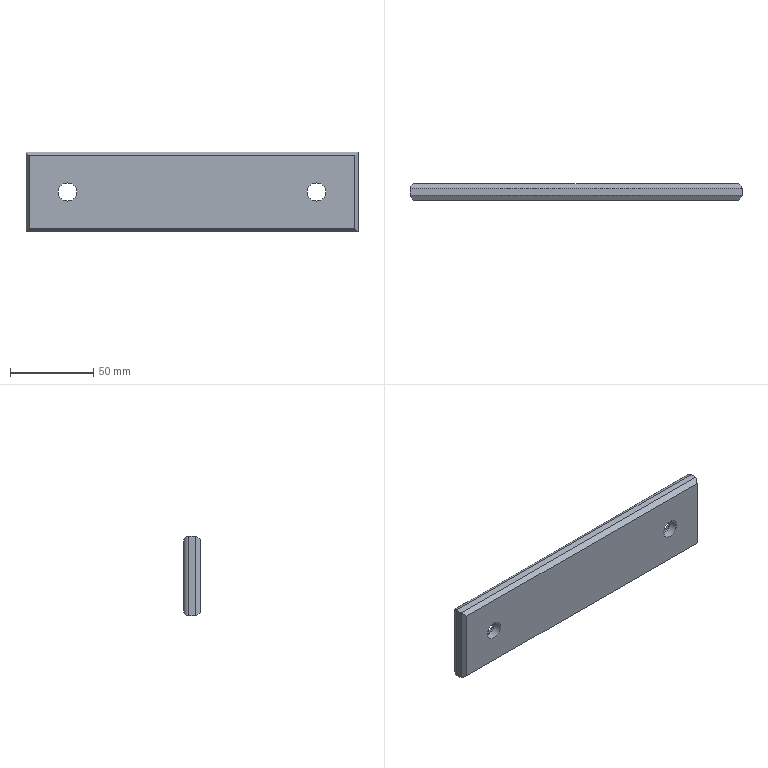Part | NX | features solid 2 | 1 solid | 22 faces | box 200 x 10 x 48 mm | volume 90126 mm3 | plane 12 | cylinder 8 | torus 2 | commonest cylinder face diameters 6 x4 11 x2 17.5 x2
STEP:
#1=CARTESIAN_POINT('',(310.,367.,141.));
#2=VERTEX_POINT('',#1);
#3=CARTESIAN_POINT('',(310.,363.,141.));
#4=VERTEX_POINT('',#3);
#5=CARTESIAN_POINT('',(310.,370.,141.));
#6=DIRECTION('',(0.,-1.,0.));
#7=VECTOR('',#6,1000.);
#8=LINE('',#5,#7);
#9=EDGE_CURVE('',#2,#4,#8,.T.);
#10=ORIENTED_EDGE('',*,*,#9,.T.);
#11=CARTESIAN_POINT('',(110.,363.,141.));
#12=VERTEX_POINT('',#11);
#13=CARTESIAN_POINT('',(110.,363.,141.));
#14=DIRECTION('',(-1.,0.,0.));
#15=VECTOR('',#14,1000.);
#16=LINE('',#13,#15);
#17=EDGE_CURVE('',#4,#12,#16,.T.);
#18=ORIENTED_EDGE('',*,*,#17,.T.);
#19=CARTESIAN_POINT('',(110.,367.,141.));
#20=VERTEX_POINT('',#19);
#21=CARTESIAN_POINT('',(110.,370.,141.));
#22=DIRECTION('',(0.,-1.,0.));
#23=VECTOR('',#22,1000.);
#24=LINE('',#21,#23);
#25=EDGE_CURVE('',#20,#12,#24,.T.);
#26=ORIENTED_EDGE('',*,*,#25,.F.);
#27=CARTESIAN_POINT('',(310.,367.,141.));
#28=DIRECTION('',(-1.,0.,0.));
#29=VECTOR('',#28,1000.);
#30=LINE('',#27,#29);
#31=EDGE_CURVE('',#20,#2,#30,.F.);
#32=ORIENTED_EDGE('',*,*,#31,.T.);
#33=EDGE_LOOP('',(#10,#18,#26,#32));
#34=FACE_BOUND('',#33,.T.);
#35=CARTESIAN_POINT('',(310.,370.,141.));
#36=DIRECTION('',(0.,0.,1.));
#37=DIRECTION('',(-1.,0.,0.));
#38=AXIS2_PLACEMENT_3D('',#35,#36,#37);
#39=PLANE('',#38);
#40=ADVANCED_FACE('',(#34),#39,.F.);
#41=ORIENTED_EDGE('',*,*,#25,.T.);
#42=CARTESIAN_POINT('',(110.,363.,189.));
#43=VERTEX_POINT('',#42);
#44=CARTESIAN_POINT('',(110.,363.,190.));
#45=DIRECTION('',(0.,0.,1.));
#46=VECTOR('',#45,1000.);
#47=LINE('',#44,#46);
#48=EDGE_CURVE('',#12,#43,#47,.T.);
#49=ORIENTED_EDGE('',*,*,#48,.T.);
#50=CARTESIAN_POINT('',(110.,367.,189.));
#51=VERTEX_POINT('',#50);
#52=CARTESIAN_POINT('',(110.,370.,189.));
#53=DIRECTION('',(0.,-1.,0.));
#54=VECTOR('',#53,1000.);
#55=LINE('',#52,#54);
#56=EDGE_CURVE('',#51,#43,#55,.T.);
#57=ORIENTED_EDGE('',*,*,#56,.F.);
#58=CARTESIAN_POINT('',(110.,367.,141.));
#59=DIRECTION('',(0.,0.,-1.));
#60=VECTOR('',#59,1000.);
#61=LINE('',#58,#60);
#62=EDGE_CURVE('',#51,#20,#61,.T.);
#63=ORIENTED_EDGE('',*,*,#62,.T.);
#64=EDGE_LOOP('',(#41,#49,#57,#63));
#65=FACE_BOUND('',#64,.T.);
#66=CARTESIAN_POINT('',(110.,370.,190.));
#67=DIRECTION('',(-1.,0.,0.));
#68=DIRECTION('',(0.,0.,-1.));
#69=AXIS2_PLACEMENT_3D('',#66,#67,#68);
#70=PLANE('',#69);
#71=ADVANCED_FACE('',(#65),#70,.T.);
#72=ORIENTED_EDGE('',*,*,#56,.T.);
#73=CARTESIAN_POINT('',(310.,363.,189.));
#74=VERTEX_POINT('',#73);
#75=CARTESIAN_POINT('',(310.,363.,189.));
#76=DIRECTION('',(1.,0.,0.));
#77=VECTOR('',#76,1000.);
#78=LINE('',#75,#77);
#79=EDGE_CURVE('',#43,#74,#78,.T.);
#80=ORIENTED_EDGE('',*,*,#79,.T.);
#81=CARTESIAN_POINT('',(310.,367.,189.));
#82=VERTEX_POINT('',#81);
#83=CARTESIAN_POINT('',(310.,370.,189.));
#84=DIRECTION('',(0.,-1.,0.));
#85=VECTOR('',#84,1000.);
#86=LINE('',#83,#85);
#87=EDGE_CURVE('',#82,#74,#86,.T.);
#88=ORIENTED_EDGE('',*,*,#87,.F.);
#89=CARTESIAN_POINT('',(110.,367.,189.));
#90=DIRECTION('',(-1.,0.,0.));
#91=VECTOR('',#90,1000.);
#92=LINE('',#89,#91);
#93=EDGE_CURVE('',#82,#51,#92,.T.);
#94=ORIENTED_EDGE('',*,*,#93,.T.);
#95=EDGE_LOOP('',(#72,#80,#88,#94));
#96=FACE_BOUND('',#95,.T.);
#97=CARTESIAN_POINT('',(310.,370.,189.));
#98=DIRECTION('',(0.,0.,1.));
#99=DIRECTION('',(-1.,0.,0.));
#100=AXIS2_PLACEMENT_3D('',#97,#98,#99);
#101=PLANE('',#100);
#102=ADVANCED_FACE('',(#96),#101,.T.);
#103=ORIENTED_EDGE('',*,*,#87,.T.);
#104=CARTESIAN_POINT('',(310.,363.,141.));
#105=DIRECTION('',(0.,0.,-1.));
#106=VECTOR('',#105,1000.);
#107=LINE('',#104,#106);
#108=EDGE_CURVE('',#74,#4,#107,.T.);
#109=ORIENTED_EDGE('',*,*,#108,.T.);
#110=ORIENTED_EDGE('',*,*,#9,.F.);
#111=CARTESIAN_POINT('',(310.,367.,190.));
#112=DIRECTION('',(0.,0.,-1.));
#113=VECTOR('',#112,1000.);
#114=LINE('',#111,#113);
#115=EDGE_CURVE('',#2,#82,#114,.F.);
#116=ORIENTED_EDGE('',*,*,#115,.T.);
#117=EDGE_LOOP('',(#103,#109,#110,#116));
#118=FACE_BOUND('',#117,.T.);
#119=CARTESIAN_POINT('',(310.,370.,190.));
#120=DIRECTION('',(-1.,0.,0.));
#121=DIRECTION('',(0.,0.,-1.));
#122=AXIS2_PLACEMENT_3D('',#119,#120,#121);
#123=PLANE('',#122);
#124=ADVANCED_FACE('',(#118),#123,.F.);
#125=CARTESIAN_POINT('',(113.,370.,186.));
#126=VERTEX_POINT('',#125);
#127=CARTESIAN_POINT('',(307.,370.,186.));
#128=VERTEX_POINT('',#127);
#129=CARTESIAN_POINT('',(310.,370.,186.));
#130=DIRECTION('',(-1.,0.,0.));
#131=VECTOR('',#130,1000.);
#132=LINE('',#129,#131);
#133=EDGE_CURVE('',#126,#128,#132,.F.);
#134=ORIENTED_EDGE('',*,*,#133,.T.);
#135=CARTESIAN_POINT('',(307.,370.,144.));
#136=VERTEX_POINT('',#135);
#137=CARTESIAN_POINT('',(307.,370.,190.));
#138=DIRECTION('',(0.,0.,-1.));
#139=VECTOR('',#138,1000.);
#140=LINE('',#137,#139);
#141=EDGE_CURVE('',#128,#136,#140,.T.);
#142=ORIENTED_EDGE('',*,*,#141,.T.);
#143=CARTESIAN_POINT('',(113.,370.,144.));
#144=VERTEX_POINT('',#143);
#145=CARTESIAN_POINT('',(310.,370.,144.));
#146=DIRECTION('',(-1.,0.,0.));
#147=VECTOR('',#146,1000.);
#148=LINE('',#145,#147);
#149=EDGE_CURVE('',#136,#144,#148,.T.);
#150=ORIENTED_EDGE('',*,*,#149,.T.);
#151=CARTESIAN_POINT('',(113.,370.,189.));
#152=DIRECTION('',(0.,0.,-1.));
#153=VECTOR('',#152,1000.);
#154=LINE('',#151,#153);
#155=EDGE_CURVE('',#144,#126,#154,.F.);
#156=ORIENTED_EDGE('',*,*,#155,.T.);
#157=EDGE_LOOP('',(#134,#142,#150,#156));
#158=FACE_BOUND('',#157,.T.);
#159=CARTESIAN_POINT('',(285.,370.,154.25));
#160=VERTEX_POINT('',#159);
#161=CARTESIAN_POINT('',(285.,370.,165.));
#162=DIRECTION('',(0.,-1.,0.));
#163=DIRECTION('',(0.,0.,-1.));
#164=AXIS2_PLACEMENT_3D('',#161,#162,#163);
#165=CIRCLE('',#164,10.75);
#166=EDGE_CURVE('',#160,#160,#165,.T.);
#167=ORIENTED_EDGE('',*,*,#166,.T.);
#168=EDGE_LOOP('',(#167));
#169=FACE_BOUND('',#168,.T.);
#170=CARTESIAN_POINT('',(135.,370.,154.25));
#171=VERTEX_POINT('',#170);
#172=CARTESIAN_POINT('',(135.,370.,165.));
#173=DIRECTION('',(0.,-1.,0.));
#174=DIRECTION('',(0.,0.,-1.));
#175=AXIS2_PLACEMENT_3D('',#172,#173,#174);
#176=CIRCLE('',#175,10.75);
#177=EDGE_CURVE('',#171,#171,#176,.T.);
#178=ORIENTED_EDGE('',*,*,#177,.T.);
#179=EDGE_LOOP('',(#178));
#180=FACE_BOUND('',#179,.T.);
#181=CARTESIAN_POINT('',(310.,370.,190.));
#182=DIRECTION('',(0.,-1.,0.));
#183=DIRECTION('',(0.,0.,-1.));
#184=AXIS2_PLACEMENT_3D('',#181,#182,#183);
#185=PLANE('',#184);
#186=ADVANCED_FACE('',(#158,#169,#180),#185,.F.);
#187=CARTESIAN_POINT('',(112.,360.,143.));
#188=VERTEX_POINT('',#187);
#189=CARTESIAN_POINT('',(308.,360.,143.));
#190=VERTEX_POINT('',#189);
#191=CARTESIAN_POINT('',(310.,360.,143.));
#192=DIRECTION('',(1.,0.,0.));
#193=VECTOR('',#192,1000.);
#194=LINE('',#191,#193);
#195=EDGE_CURVE('',#188,#190,#194,.T.);
#196=ORIENTED_EDGE('',*,*,#195,.T.);
#197=CARTESIAN_POINT('',(308.,360.,187.));
#198=VERTEX_POINT('',#197);
#199=CARTESIAN_POINT('',(308.,360.,189.));
#200=DIRECTION('',(0.,0.,1.));
#201=VECTOR('',#200,1000.);
#202=LINE('',#199,#201);
#203=EDGE_CURVE('',#190,#198,#202,.T.);
#204=ORIENTED_EDGE('',*,*,#203,.T.);
#205=CARTESIAN_POINT('',(112.,360.,187.));
#206=VERTEX_POINT('',#205);
#207=CARTESIAN_POINT('',(310.,360.,187.));
#208=DIRECTION('',(-1.,0.,0.));
#209=VECTOR('',#208,1000.);
#210=LINE('',#207,#209);
#211=EDGE_CURVE('',#198,#206,#210,.T.);
#212=ORIENTED_EDGE('',*,*,#211,.T.);
#213=CARTESIAN_POINT('',(112.,360.,190.));
#214=DIRECTION('',(0.,0.,-1.));
#215=VECTOR('',#214,1000.);
#216=LINE('',#213,#215);
#217=EDGE_CURVE('',#206,#188,#216,.T.);
#218=ORIENTED_EDGE('',*,*,#217,.T.);
#219=EDGE_LOOP('',(#196,#204,#212,#218));
#220=FACE_BOUND('',#219,.T.);
#221=CARTESIAN_POINT('',(135.,360.,159.5));
#222=VERTEX_POINT('',#221);
#223=CARTESIAN_POINT('',(135.,360.,165.));
#224=DIRECTION('',(0.,-1.,0.));
#225=DIRECTION('',(0.,0.,-1.));
#226=AXIS2_PLACEMENT_3D('',#223,#224,#225);
#227=CIRCLE('',#226,5.5);
#228=EDGE_CURVE('',#222,#222,#227,.T.);
#229=ORIENTED_EDGE('',*,*,#228,.F.);
#230=EDGE_LOOP('',(#229));
#231=FACE_BOUND('',#230,.T.);
#232=CARTESIAN_POINT('',(285.,360.,159.5));
#233=VERTEX_POINT('',#232);
#234=CARTESIAN_POINT('',(285.,360.,165.));
#235=DIRECTION('',(0.,-1.,0.));
#236=DIRECTION('',(0.,0.,-1.));
#237=AXIS2_PLACEMENT_3D('',#234,#235,#236);
#238=CIRCLE('',#237,5.5);
#239=EDGE_CURVE('',#233,#233,#238,.T.);
#240=ORIENTED_EDGE('',*,*,#239,.F.);
#241=EDGE_LOOP('',(#240));
#242=FACE_BOUND('',#241,.T.);
#243=CARTESIAN_POINT('',(310.,360.,190.));
#244=DIRECTION('',(0.,-1.,0.));
#245=DIRECTION('',(0.,0.,-1.));
#246=AXIS2_PLACEMENT_3D('',#243,#244,#245);
#247=PLANE('',#246);
#248=ADVANCED_FACE('',(#220,#231,#242),#247,.T.);
#249=ORIENTED_EDGE('',*,*,#239,.T.);
#250=EDGE_LOOP('',(#249));
#251=FACE_BOUND('',#250,.T.);
#252=CARTESIAN_POINT('',(285.,365.,159.5));
#253=VERTEX_POINT('',#252);
#254=CARTESIAN_POINT('',(285.,365.,165.));
#255=DIRECTION('',(0.,-1.,0.));
#256=DIRECTION('',(0.,0.,-1.));
#257=AXIS2_PLACEMENT_3D('',#254,#255,#256);
#258=CIRCLE('',#257,5.5);
#259=EDGE_CURVE('',#253,#253,#258,.T.);
#260=ORIENTED_EDGE('',*,*,#259,.F.);
#261=EDGE_LOOP('',(#260));
#262=FACE_BOUND('',#261,.T.);
#263=CARTESIAN_POINT('',(285.,360.,165.));
#264=DIRECTION('',(0.,-1.,0.));
#265=DIRECTION('',(0.,0.,-1.));
#266=AXIS2_PLACEMENT_3D('',#263,#264,#265);
#267=CYLINDRICAL_SURFACE('',#266,5.5);
#268=ADVANCED_FACE('',(#251,#262),#267,.F.);
#269=ORIENTED_EDGE('',*,*,#259,.T.);
#270=EDGE_LOOP('',(#269));
#271=FACE_BOUND('',#270,.T.);
#272=CARTESIAN_POINT('',(285.,365.,156.25));
#273=VERTEX_POINT('',#272);
#274=CARTESIAN_POINT('',(285.,365.,165.));
#275=DIRECTION('',(0.,-1.,0.));
#276=DIRECTION('',(0.,0.,-1.));
#277=AXIS2_PLACEMENT_3D('',#274,#275,#276);
#278=CIRCLE('',#277,8.75);
#279=EDGE_CURVE('',#273,#273,#278,.T.);
#280=ORIENTED_EDGE('',*,*,#279,.F.);
#281=EDGE_LOOP('',(#280));
#282=FACE_BOUND('',#281,.T.);
#283=CARTESIAN_POINT('',(285.,365.,165.));
#284=DIRECTION('',(0.,-1.,0.));
#285=DIRECTION('',(0.,0.,-1.));
#286=AXIS2_PLACEMENT_3D('',#283,#284,#285);
#287=PLANE('',#286);
#288=ADVANCED_FACE('',(#271,#282),#287,.F.);
#289=CARTESIAN_POINT('',(285.,368.,156.25));
#290=VERTEX_POINT('',#289);
#291=CARTESIAN_POINT('',(285.,368.,165.));
#292=DIRECTION('',(0.,-1.,0.));
#293=DIRECTION('',(0.,0.,-1.));
#294=AXIS2_PLACEMENT_3D('',#291,#292,#293);
#295=CIRCLE('',#294,8.75);
#296=EDGE_CURVE('',#290,#290,#295,.F.);
#297=ORIENTED_EDGE('',*,*,#296,.T.);
#298=EDGE_LOOP('',(#297));
#299=FACE_BOUND('',#298,.T.);
#300=ORIENTED_EDGE('',*,*,#279,.T.);
#301=EDGE_LOOP('',(#300));
#302=FACE_BOUND('',#301,.T.);
#303=CARTESIAN_POINT('',(285.,370.,165.));
#304=DIRECTION('',(0.,-1.,0.));
#305=DIRECTION('',(0.,0.,-1.));
#306=AXIS2_PLACEMENT_3D('',#303,#304,#305);
#307=CYLINDRICAL_SURFACE('',#306,8.75);
#308=ADVANCED_FACE('',(#299,#302),#307,.F.);
#309=ORIENTED_EDGE('',*,*,#228,.T.);
#310=EDGE_LOOP('',(#309));
#311=FACE_BOUND('',#310,.T.);
#312=CARTESIAN_POINT('',(135.,365.,159.5));
#313=VERTEX_POINT('',#312);
#314=CARTESIAN_POINT('',(135.,365.,165.));
#315=DIRECTION('',(0.,-1.,0.));
#316=DIRECTION('',(0.,0.,-1.));
#317=AXIS2_PLACEMENT_3D('',#314,#315,#316);
#318=CIRCLE('',#317,5.5);
#319=EDGE_CURVE('',#313,#313,#318,.T.);
#320=ORIENTED_EDGE('',*,*,#319,.F.);
#321=EDGE_LOOP('',(#320));
#322=FACE_BOUND('',#321,.T.);
#323=CARTESIAN_POINT('',(135.,360.,165.));
#324=DIRECTION('',(0.,-1.,0.));
#325=DIRECTION('',(0.,0.,-1.));
#326=AXIS2_PLACEMENT_3D('',#323,#324,#325);
#327=CYLINDRICAL_SURFACE('',#326,5.5);
#328=ADVANCED_FACE('',(#311,#322),#327,.F.);
#329=ORIENTED_EDGE('',*,*,#319,.T.);
#330=EDGE_LOOP('',(#329));
#331=FACE_BOUND('',#330,.T.);
#332=CARTESIAN_POINT('',(135.,365.,156.25));
#333=VERTEX_POINT('',#332);
#334=CARTESIAN_POINT('',(135.,365.,165.));
#335=DIRECTION('',(0.,-1.,0.));
#336=DIRECTION('',(0.,0.,-1.));
#337=AXIS2_PLACEMENT_3D('',#334,#335,#336);
#338=CIRCLE('',#337,8.75);
#339=EDGE_CURVE('',#333,#333,#338,.T.);
#340=ORIENTED_EDGE('',*,*,#339,.F.);
#341=EDGE_LOOP('',(#340));
#342=FACE_BOUND('',#341,.T.);
#343=CARTESIAN_POINT('',(135.,365.,165.));
#344=DIRECTION('',(0.,-1.,0.));
#345=DIRECTION('',(0.,0.,-1.));
#346=AXIS2_PLACEMENT_3D('',#343,#344,#345);
#347=PLANE('',#346);
#348=ADVANCED_FACE('',(#331,#342),#347,.F.);
#349=CARTESIAN_POINT('',(135.,368.,156.25));
#350=VERTEX_POINT('',#349);
#351=CARTESIAN_POINT('',(135.,368.,165.));
#352=DIRECTION('',(0.,-1.,0.));
#353=DIRECTION('',(0.,0.,-1.));
#354=AXIS2_PLACEMENT_3D('',#351,#352,#353);
#355=CIRCLE('',#354,8.75);
#356=EDGE_CURVE('',#350,#350,#355,.F.);
#357=ORIENTED_EDGE('',*,*,#356,.T.);
#358=EDGE_LOOP('',(#357));
#359=FACE_BOUND('',#358,.T.);
#360=ORIENTED_EDGE('',*,*,#339,.T.);
#361=EDGE_LOOP('',(#360));
#362=FACE_BOUND('',#361,.T.);
#363=CARTESIAN_POINT('',(135.,370.,165.));
#364=DIRECTION('',(0.,-1.,0.));
#365=DIRECTION('',(0.,0.,-1.));
#366=AXIS2_PLACEMENT_3D('',#363,#364,#365);
#367=CYLINDRICAL_SURFACE('',#366,8.75);
#368=ADVANCED_FACE('',(#359,#362),#367,.F.);
#369=ORIENTED_EDGE('',*,*,#296,.F.);
#370=EDGE_LOOP('',(#369));
#371=FACE_BOUND('',#370,.T.);
#372=ORIENTED_EDGE('',*,*,#166,.F.);
#373=EDGE_LOOP('',(#372));
#374=FACE_BOUND('',#373,.T.);
#375=CARTESIAN_POINT('',(285.,368.,165.));
#376=DIRECTION('',(0.,-1.,0.));
#377=DIRECTION('',(0.,0.,-1.));
#378=AXIS2_PLACEMENT_3D('',#375,#376,#377);
#379=TOROIDAL_SURFACE('',#378,10.75,2.);
#380=ADVANCED_FACE('',(#371,#374),#379,.T.);
#381=ORIENTED_EDGE('',*,*,#356,.F.);
#382=EDGE_LOOP('',(#381));
#383=FACE_BOUND('',#382,.T.);
#384=ORIENTED_EDGE('',*,*,#177,.F.);
#385=EDGE_LOOP('',(#384));
#386=FACE_BOUND('',#385,.T.);
#387=CARTESIAN_POINT('',(135.,368.,165.));
#388=DIRECTION('',(0.,-1.,0.));
#389=DIRECTION('',(0.,0.,-1.));
#390=AXIS2_PLACEMENT_3D('',#387,#388,#389);
#391=TOROIDAL_SURFACE('',#390,10.75,2.);
#392=ADVANCED_FACE('',(#383,#386),#391,.T.);
#393=CARTESIAN_POINT('',(113.,367.,144.));
#394=DIRECTION('',(-0.7071,0.,0.7071));
#395=DIRECTION('',(0.7071,0.,0.7071));
#396=AXIS2_PLACEMENT_3D('',#393,#394,#395);
#397=ELLIPSE('',#396,4.243,3.);
#398=EDGE_CURVE('',#20,#144,#397,.F.);
#399=ORIENTED_EDGE('',*,*,#398,.F.);
#400=ORIENTED_EDGE('',*,*,#62,.F.);
#401=CARTESIAN_POINT('',(113.,367.,186.));
#402=DIRECTION('',(0.7071,0.,0.7071));
#403=DIRECTION('',(0.7071,0.,-0.7071));
#404=AXIS2_PLACEMENT_3D('',#401,#402,#403);
#405=ELLIPSE('',#404,4.243,3.);
#406=EDGE_CURVE('',#126,#51,#405,.T.);
#407=ORIENTED_EDGE('',*,*,#406,.F.);
#408=ORIENTED_EDGE('',*,*,#155,.F.);
#409=EDGE_LOOP('',(#399,#400,#407,#408));
#410=FACE_BOUND('',#409,.T.);
#411=CARTESIAN_POINT('',(113.,367.,190.));
#412=DIRECTION('',(0.,0.,1.));
#413=DIRECTION('',(0.,-1.,0.));
#414=AXIS2_PLACEMENT_3D('',#411,#412,#413);
#415=CYLINDRICAL_SURFACE('',#414,3.);
#416=ADVANCED_FACE('',(#410),#415,.T.);
#417=ORIENTED_EDGE('',*,*,#406,.T.);
#418=ORIENTED_EDGE('',*,*,#93,.F.);
#419=CARTESIAN_POINT('',(307.,367.,186.));
#420=DIRECTION('',(0.7071,0.,-0.7071));
#421=DIRECTION('',(0.7071,0.,0.7071));
#422=AXIS2_PLACEMENT_3D('',#419,#420,#421);
#423=ELLIPSE('',#422,4.243,3.);
#424=EDGE_CURVE('',#128,#82,#423,.T.);
#425=ORIENTED_EDGE('',*,*,#424,.F.);
#426=ORIENTED_EDGE('',*,*,#133,.F.);
#427=EDGE_LOOP('',(#417,#418,#425,#426));
#428=FACE_BOUND('',#427,.T.);
#429=CARTESIAN_POINT('',(310.,367.,186.));
#430=DIRECTION('',(1.,0.,0.));
#431=DIRECTION('',(0.,0.,1.));
#432=AXIS2_PLACEMENT_3D('',#429,#430,#431);
#433=CYLINDRICAL_SURFACE('',#432,3.);
#434=ADVANCED_FACE('',(#428),#433,.T.);
#435=ORIENTED_EDGE('',*,*,#398,.T.);
#436=ORIENTED_EDGE('',*,*,#149,.F.);
#437=CARTESIAN_POINT('',(307.,367.,144.));
#438=DIRECTION('',(-0.7071,0.,-0.7071));
#439=DIRECTION('',(-0.7071,0.,0.7071));
#440=AXIS2_PLACEMENT_3D('',#437,#438,#439);
#441=ELLIPSE('',#440,4.243,3.);
#442=EDGE_CURVE('',#2,#136,#441,.F.);
#443=ORIENTED_EDGE('',*,*,#442,.F.);
#444=ORIENTED_EDGE('',*,*,#31,.F.);
#445=EDGE_LOOP('',(#435,#436,#443,#444));
#446=FACE_BOUND('',#445,.T.);
#447=CARTESIAN_POINT('',(310.,367.,144.));
#448=DIRECTION('',(-1.,0.,0.));
#449=DIRECTION('',(0.,0.,-1.));
#450=AXIS2_PLACEMENT_3D('',#447,#448,#449);
#451=CYLINDRICAL_SURFACE('',#450,3.);
#452=ADVANCED_FACE('',(#446),#451,.T.);
#453=ORIENTED_EDGE('',*,*,#424,.T.);
#454=ORIENTED_EDGE('',*,*,#115,.F.);
#455=ORIENTED_EDGE('',*,*,#442,.T.);
#456=ORIENTED_EDGE('',*,*,#141,.F.);
#457=EDGE_LOOP('',(#453,#454,#455,#456));
#458=FACE_BOUND('',#457,.T.);
#459=CARTESIAN_POINT('',(307.,367.,190.));
#460=DIRECTION('',(0.,0.,-1.));
#461=DIRECTION('',(0.,1.,0.));
#462=AXIS2_PLACEMENT_3D('',#459,#460,#461);
#463=CYLINDRICAL_SURFACE('',#462,3.);
#464=ADVANCED_FACE('',(#458),#463,.T.);
#465=CARTESIAN_POINT('',(123.059,343.412,154.059));
#466=DIRECTION('',(-0.4851,0.7276,-0.4851));
#467=VECTOR('',#466,1000.);
#468=LINE('',#465,#467);
#469=EDGE_CURVE('',#188,#12,#468,.T.);
#470=ORIENTED_EDGE('',*,*,#469,.F.);
#471=ORIENTED_EDGE('',*,*,#217,.F.);
#472=CARTESIAN_POINT('',(158.588,290.118,140.412));
#473=DIRECTION('',(0.4851,-0.7276,-0.4851));
#474=VECTOR('',#473,1000.);
#475=LINE('',#472,#474);
#476=EDGE_CURVE('',#43,#206,#475,.T.);
#477=ORIENTED_EDGE('',*,*,#476,.F.);
#478=ORIENTED_EDGE('',*,*,#48,.F.);
#479=EDGE_LOOP('',(#470,#471,#477,#478));
#480=FACE_BOUND('',#479,.T.);
#481=CARTESIAN_POINT('',(112.,360.,190.));
#482=DIRECTION('',(0.8321,0.5547,0.));
#483=DIRECTION('',(-0.5547,0.8321,0.));
#484=AXIS2_PLACEMENT_3D('',#481,#482,#483);
#485=PLANE('',#484);
#486=ADVANCED_FACE('',(#480),#485,.F.);
#487=ORIENTED_EDGE('',*,*,#476,.T.);
#488=ORIENTED_EDGE('',*,*,#211,.F.);
#489=CARTESIAN_POINT('',(308.471,360.706,187.471));
#490=DIRECTION('',(-0.4851,-0.7276,-0.4851));
#491=VECTOR('',#490,1000.);
#492=LINE('',#489,#491);
#493=EDGE_CURVE('',#74,#198,#492,.T.);
#494=ORIENTED_EDGE('',*,*,#493,.F.);
#495=ORIENTED_EDGE('',*,*,#79,.F.);
#496=EDGE_LOOP('',(#487,#488,#494,#495));
#497=FACE_BOUND('',#496,.T.);
#498=CARTESIAN_POINT('',(310.,360.,187.));
#499=DIRECTION('',(0.,0.5547,-0.8321));
#500=DIRECTION('',(0.,0.8321,0.5547));
#501=AXIS2_PLACEMENT_3D('',#498,#499,#500);
#502=PLANE('',#501);
#503=ADVANCED_FACE('',(#497),#502,.F.);
#504=ORIENTED_EDGE('',*,*,#469,.T.);
#505=ORIENTED_EDGE('',*,*,#17,.F.);
#506=CARTESIAN_POINT('',(310.,363.,141.));
#507=DIRECTION('',(-0.4851,-0.7276,0.4851));
#508=VECTOR('',#507,1000.);
#509=LINE('',#506,#508);
#510=EDGE_CURVE('',#190,#4,#509,.F.);
#511=ORIENTED_EDGE('',*,*,#510,.F.);
#512=ORIENTED_EDGE('',*,*,#195,.F.);
#513=EDGE_LOOP('',(#504,#505,#511,#512));
#514=FACE_BOUND('',#513,.T.);
#515=CARTESIAN_POINT('',(310.,363.,141.));
#516=DIRECTION('',(0.,-0.5547,-0.8321));
#517=DIRECTION('',(0.,0.8321,-0.5547));
#518=AXIS2_PLACEMENT_3D('',#515,#516,#517);
#519=PLANE('',#518);
#520=ADVANCED_FACE('',(#514),#519,.T.);
#521=ORIENTED_EDGE('',*,*,#493,.T.);
#522=ORIENTED_EDGE('',*,*,#203,.F.);
#523=ORIENTED_EDGE('',*,*,#510,.T.);
#524=ORIENTED_EDGE('',*,*,#108,.F.);
#525=EDGE_LOOP('',(#521,#522,#523,#524));
#526=FACE_BOUND('',#525,.T.);
#527=CARTESIAN_POINT('',(310.,363.,190.));
#528=DIRECTION('',(0.8321,-0.5547,0.));
#529=DIRECTION('',(0.5547,0.8321,0.));
#530=AXIS2_PLACEMENT_3D('',#527,#528,#529);
#531=PLANE('',#530);
#532=ADVANCED_FACE('',(#526),#531,.T.);
#533=CLOSED_SHELL('',(#40,#71,#102,#124,#186,#248,#268,#288,#308,#328,#348,#368,#380,#392,#416,#434,#452,#464,#486,#503,#520,#532));
#534=MANIFOLD_SOLID_BREP('',#533);
#535=(LENGTH_UNIT()NAMED_UNIT(*)SI_UNIT(.MILLI.,.METRE.));
#536=UNCERTAINTY_MEASURE_WITH_UNIT(LENGTH_MEASURE(0.00001),#535,'','');
#537=(NAMED_UNIT(*)PLANE_ANGLE_UNIT()SI_UNIT($,.RADIAN.));
#538=(NAMED_UNIT(*)SI_UNIT($,.STERADIAN.)SOLID_ANGLE_UNIT());
#539=(GEOMETRIC_REPRESENTATION_CONTEXT(3)GLOBAL_UNCERTAINTY_ASSIGNED_CONTEXT((#536))GLOBAL_UNIT_ASSIGNED_CONTEXT((#535,#537,#538))REPRESENTATION_CONTEXT('',''));
#540=ADVANCED_BREP_SHAPE_REPRESENTATION('',(#534),#539);